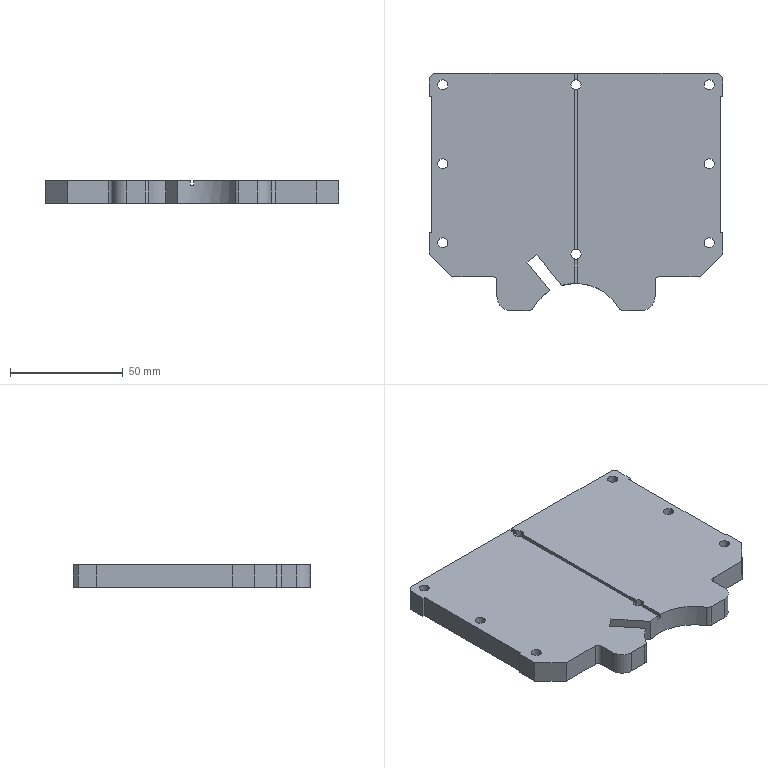Part | SolidWorks | features ICE 5, Fillet 3, Chamfer 2, HoleWzd 2, Extrusion 1 | 1 solid | 88 faces | box 130 x 105 x 10 mm | volume 118021 mm3 | plane 44 | cylinder 42 | cone 2 | commonest cylinder face diameters 4.5 x16 8 x16 4 x4 2.5 x2 12 x2 44 x2